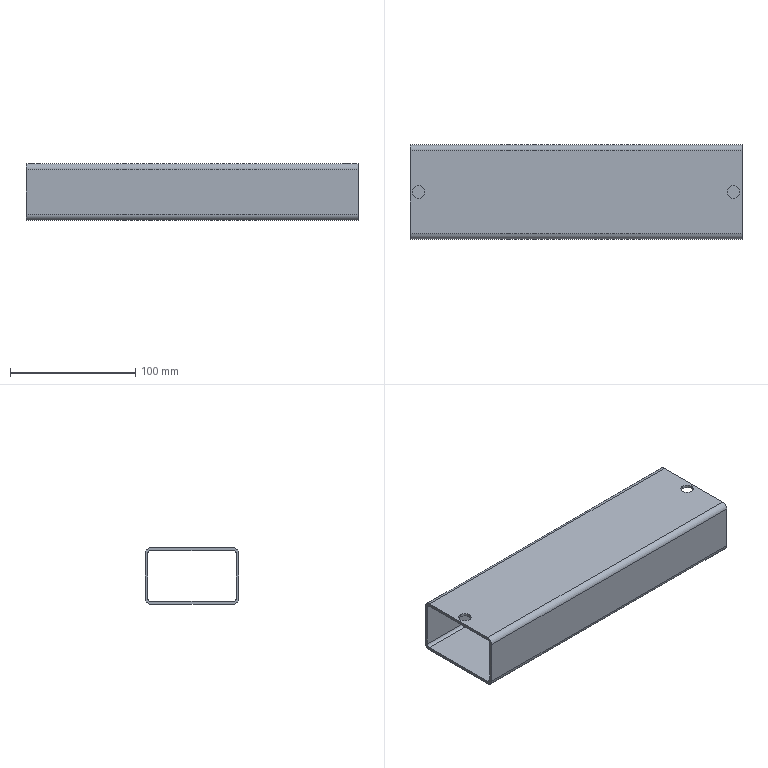Part | STEP file | [05]-1 | 1 solid | 22 faces | box 265 x 75 x 45 mm | volume 136701 mm3 | cylinder 12 | plane 10 | commonest cylinder face diameters 4.6 x4 9.2 x4 10 x4
STEP:
#1=CARTESIAN_POINT('',(278.,42.5,45.));
#2=VERTEX_POINT('',#1);
#3=CARTESIAN_POINT('',(278.,32.5,45.));
#4=VERTEX_POINT('',#3);
#5=CARTESIAN_POINT('',(278.,37.5,45.));
#6=DIRECTION('',(0.,0.,-1.));
#7=DIRECTION('',(0.,-1.,0.));
#8=AXIS2_PLACEMENT_3D('',#5,#6,#7);
#9=CIRCLE('',#8,5.);
#10=EDGE_CURVE('',#2,#4,#9,.T.);
#11=ORIENTED_EDGE('',*,*,#10,.F.);
#12=CARTESIAN_POINT('',(278.,42.5,42.7));
#13=VERTEX_POINT('',#12);
#14=CARTESIAN_POINT('',(278.,42.5,45.));
#15=DIRECTION('',(0.,0.,-1.));
#16=VECTOR('',#15,1000.);
#17=LINE('',#14,#16);
#18=EDGE_CURVE('',#2,#13,#17,.T.);
#19=ORIENTED_EDGE('',*,*,#18,.T.);
#20=CARTESIAN_POINT('',(278.,32.5,42.7));
#21=VERTEX_POINT('',#20);
#22=CARTESIAN_POINT('',(278.,37.5,42.7));
#23=DIRECTION('',(0.,0.,1.));
#24=DIRECTION('',(0.,1.,0.));
#25=AXIS2_PLACEMENT_3D('',#22,#23,#24);
#26=CIRCLE('',#25,5.);
#27=EDGE_CURVE('',#21,#13,#26,.T.);
#28=ORIENTED_EDGE('',*,*,#27,.F.);
#29=CARTESIAN_POINT('',(278.,32.5,45.));
#30=DIRECTION('',(0.,0.,-1.));
#31=VECTOR('',#30,1000.);
#32=LINE('',#29,#31);
#33=EDGE_CURVE('',#4,#21,#32,.T.);
#34=ORIENTED_EDGE('',*,*,#33,.F.);
#35=EDGE_LOOP('',(#11,#19,#28,#34));
#36=FACE_OUTER_BOUND('',#35,.T.);
#37=CARTESIAN_POINT('',(278.,37.5,45.));
#38=DIRECTION('',(0.,0.,-1.));
#39=DIRECTION('',(0.,-1.,0.));
#40=AXIS2_PLACEMENT_3D('',#37,#38,#39);
#41=CYLINDRICAL_SURFACE('',#40,5.);
#42=ADVANCED_FACE('',(#36),#41,.F.);
#43=CARTESIAN_POINT('',(27.,42.5,45.));
#44=VERTEX_POINT('',#43);
#45=CARTESIAN_POINT('',(27.,32.5,45.));
#46=VERTEX_POINT('',#45);
#47=CARTESIAN_POINT('',(27.,37.5,45.));
#48=DIRECTION('',(0.,0.,-1.));
#49=DIRECTION('',(0.,-1.,0.));
#50=AXIS2_PLACEMENT_3D('',#47,#48,#49);
#51=CIRCLE('',#50,5.);
#52=EDGE_CURVE('',#44,#46,#51,.T.);
#53=ORIENTED_EDGE('',*,*,#52,.F.);
#54=CARTESIAN_POINT('',(27.,42.5,42.7));
#55=VERTEX_POINT('',#54);
#56=CARTESIAN_POINT('',(27.,42.5,45.));
#57=DIRECTION('',(0.,0.,-1.));
#58=VECTOR('',#57,1000.);
#59=LINE('',#56,#58);
#60=EDGE_CURVE('',#44,#55,#59,.T.);
#61=ORIENTED_EDGE('',*,*,#60,.T.);
#62=CARTESIAN_POINT('',(27.,32.5,42.7));
#63=VERTEX_POINT('',#62);
#64=CARTESIAN_POINT('',(27.,37.5,42.7));
#65=DIRECTION('',(0.,0.,1.));
#66=DIRECTION('',(0.,1.,0.));
#67=AXIS2_PLACEMENT_3D('',#64,#65,#66);
#68=CIRCLE('',#67,5.);
#69=EDGE_CURVE('',#63,#55,#68,.T.);
#70=ORIENTED_EDGE('',*,*,#69,.F.);
#71=CARTESIAN_POINT('',(27.,32.5,45.));
#72=DIRECTION('',(0.,0.,-1.));
#73=VECTOR('',#72,1000.);
#74=LINE('',#71,#73);
#75=EDGE_CURVE('',#46,#63,#74,.T.);
#76=ORIENTED_EDGE('',*,*,#75,.F.);
#77=EDGE_LOOP('',(#53,#61,#70,#76));
#78=FACE_OUTER_BOUND('',#77,.T.);
#79=CARTESIAN_POINT('',(27.,37.5,45.));
#80=DIRECTION('',(0.,0.,-1.));
#81=DIRECTION('',(0.,-1.,0.));
#82=AXIS2_PLACEMENT_3D('',#79,#80,#81);
#83=CYLINDRICAL_SURFACE('',#82,5.);
#84=ADVANCED_FACE('',(#78),#83,.F.);
#85=CARTESIAN_POINT('',(20.,70.4,0.));
#86=VERTEX_POINT('',#85);
#87=CARTESIAN_POINT('',(20.,4.6,0.));
#88=VERTEX_POINT('',#87);
#89=CARTESIAN_POINT('',(20.,70.4,0.));
#90=DIRECTION('',(0.,-1.,0.));
#91=VECTOR('',#90,1000.);
#92=LINE('',#89,#91);
#93=EDGE_CURVE('',#86,#88,#92,.T.);
#94=ORIENTED_EDGE('',*,*,#93,.T.);
#95=CARTESIAN_POINT('',(20.,0.,4.6));
#96=VERTEX_POINT('',#95);
#97=CARTESIAN_POINT('',(20.,4.6,4.6));
#98=DIRECTION('',(-1.,0.,0.));
#99=DIRECTION('',(0.,0.,-1.));
#100=AXIS2_PLACEMENT_3D('',#97,#98,#99);
#101=CIRCLE('',#100,4.6);
#102=EDGE_CURVE('',#88,#96,#101,.T.);
#103=ORIENTED_EDGE('',*,*,#102,.T.);
#104=CARTESIAN_POINT('',(20.,0.,40.4));
#105=VERTEX_POINT('',#104);
#106=CARTESIAN_POINT('',(20.,0.,4.6));
#107=DIRECTION('',(0.,0.,1.));
#108=VECTOR('',#107,1000.);
#109=LINE('',#106,#108);
#110=EDGE_CURVE('',#96,#105,#109,.T.);
#111=ORIENTED_EDGE('',*,*,#110,.T.);
#112=CARTESIAN_POINT('',(20.,4.6,45.));
#113=VERTEX_POINT('',#112);
#114=CARTESIAN_POINT('',(20.,4.6,40.4));
#115=DIRECTION('',(-1.,0.,0.));
#116=DIRECTION('',(0.,0.,-1.));
#117=AXIS2_PLACEMENT_3D('',#114,#115,#116);
#118=CIRCLE('',#117,4.6);
#119=EDGE_CURVE('',#105,#113,#118,.T.);
#120=ORIENTED_EDGE('',*,*,#119,.T.);
#121=CARTESIAN_POINT('',(20.,70.4,45.));
#122=VERTEX_POINT('',#121);
#123=CARTESIAN_POINT('',(20.,4.6,45.));
#124=DIRECTION('',(0.,1.,0.));
#125=VECTOR('',#124,1000.);
#126=LINE('',#123,#125);
#127=EDGE_CURVE('',#113,#122,#126,.T.);
#128=ORIENTED_EDGE('',*,*,#127,.T.);
#129=CARTESIAN_POINT('',(20.,75.,40.4));
#130=VERTEX_POINT('',#129);
#131=CARTESIAN_POINT('',(20.,70.4,40.4));
#132=DIRECTION('',(-1.,0.,0.));
#133=DIRECTION('',(0.,0.,-1.));
#134=AXIS2_PLACEMENT_3D('',#131,#132,#133);
#135=CIRCLE('',#134,4.6);
#136=EDGE_CURVE('',#122,#130,#135,.T.);
#137=ORIENTED_EDGE('',*,*,#136,.T.);
#138=CARTESIAN_POINT('',(20.,75.,4.6));
#139=VERTEX_POINT('',#138);
#140=CARTESIAN_POINT('',(20.,75.,40.4));
#141=DIRECTION('',(0.,0.,-1.));
#142=VECTOR('',#141,1000.);
#143=LINE('',#140,#142);
#144=EDGE_CURVE('',#130,#139,#143,.T.);
#145=ORIENTED_EDGE('',*,*,#144,.T.);
#146=CARTESIAN_POINT('',(20.,70.4,4.6));
#147=DIRECTION('',(-1.,0.,0.));
#148=DIRECTION('',(0.,0.,-1.));
#149=AXIS2_PLACEMENT_3D('',#146,#147,#148);
#150=CIRCLE('',#149,4.6);
#151=EDGE_CURVE('',#139,#86,#150,.T.);
#152=ORIENTED_EDGE('',*,*,#151,.T.);
#153=EDGE_LOOP('',(#94,#103,#111,#120,#128,#137,#145,#152));
#154=FACE_OUTER_BOUND('',#153,.T.);
#155=CARTESIAN_POINT('',(20.,70.4,2.3));
#156=VERTEX_POINT('',#155);
#157=CARTESIAN_POINT('',(20.,4.6,2.3));
#158=VERTEX_POINT('',#157);
#159=CARTESIAN_POINT('',(20.,70.4,2.3));
#160=DIRECTION('',(0.,-1.,0.));
#161=VECTOR('',#160,1000.);
#162=LINE('',#159,#161);
#163=EDGE_CURVE('',#156,#158,#162,.T.);
#164=ORIENTED_EDGE('',*,*,#163,.F.);
#165=CARTESIAN_POINT('',(20.,72.7,4.6));
#166=VERTEX_POINT('',#165);
#167=CARTESIAN_POINT('',(20.,70.4,4.6));
#168=DIRECTION('',(-1.,0.,0.));
#169=DIRECTION('',(0.,1.,0.));
#170=AXIS2_PLACEMENT_3D('',#167,#168,#169);
#171=CIRCLE('',#170,2.3);
#172=EDGE_CURVE('',#166,#156,#171,.T.);
#173=ORIENTED_EDGE('',*,*,#172,.F.);
#174=CARTESIAN_POINT('',(20.,72.7,40.4));
#175=VERTEX_POINT('',#174);
#176=CARTESIAN_POINT('',(20.,72.7,40.4));
#177=DIRECTION('',(0.,0.,-1.));
#178=VECTOR('',#177,1000.);
#179=LINE('',#176,#178);
#180=EDGE_CURVE('',#175,#166,#179,.T.);
#181=ORIENTED_EDGE('',*,*,#180,.F.);
#182=CARTESIAN_POINT('',(20.,70.4,42.7));
#183=VERTEX_POINT('',#182);
#184=CARTESIAN_POINT('',(20.,70.4,40.4));
#185=DIRECTION('',(-1.,0.,0.));
#186=DIRECTION('',(0.,1.,0.));
#187=AXIS2_PLACEMENT_3D('',#184,#185,#186);
#188=CIRCLE('',#187,2.3);
#189=EDGE_CURVE('',#183,#175,#188,.T.);
#190=ORIENTED_EDGE('',*,*,#189,.F.);
#191=CARTESIAN_POINT('',(20.,4.6,42.7));
#192=VERTEX_POINT('',#191);
#193=CARTESIAN_POINT('',(20.,4.6,42.7));
#194=DIRECTION('',(0.,1.,0.));
#195=VECTOR('',#194,1000.);
#196=LINE('',#193,#195);
#197=EDGE_CURVE('',#192,#183,#196,.T.);
#198=ORIENTED_EDGE('',*,*,#197,.F.);
#199=CARTESIAN_POINT('',(20.,2.3,40.4));
#200=VERTEX_POINT('',#199);
#201=CARTESIAN_POINT('',(20.,4.6,40.4));
#202=DIRECTION('',(-1.,0.,0.));
#203=DIRECTION('',(0.,1.,0.));
#204=AXIS2_PLACEMENT_3D('',#201,#202,#203);
#205=CIRCLE('',#204,2.3);
#206=EDGE_CURVE('',#200,#192,#205,.T.);
#207=ORIENTED_EDGE('',*,*,#206,.F.);
#208=CARTESIAN_POINT('',(20.,2.3,4.6));
#209=VERTEX_POINT('',#208);
#210=CARTESIAN_POINT('',(20.,2.3,4.6));
#211=DIRECTION('',(0.,0.,1.));
#212=VECTOR('',#211,1000.);
#213=LINE('',#210,#212);
#214=EDGE_CURVE('',#209,#200,#213,.T.);
#215=ORIENTED_EDGE('',*,*,#214,.F.);
#216=CARTESIAN_POINT('',(20.,4.6,4.6));
#217=DIRECTION('',(-1.,0.,0.));
#218=DIRECTION('',(0.,1.,0.));
#219=AXIS2_PLACEMENT_3D('',#216,#217,#218);
#220=CIRCLE('',#219,2.3);
#221=EDGE_CURVE('',#158,#209,#220,.T.);
#222=ORIENTED_EDGE('',*,*,#221,.F.);
#223=EDGE_LOOP('',(#164,#173,#181,#190,#198,#207,#215,#222));
#224=FACE_BOUND('',#223,.T.);
#225=CARTESIAN_POINT('',(20.,4.6,4.6));
#226=DIRECTION('',(-1.,0.,0.));
#227=DIRECTION('',(0.,0.,-1.));
#228=AXIS2_PLACEMENT_3D('',#225,#226,#227);
#229=PLANE('',#228);
#230=ADVANCED_FACE('',(#154,#224),#229,.T.);
#231=CARTESIAN_POINT('',(285.,70.4,0.));
#232=VERTEX_POINT('',#231);
#233=CARTESIAN_POINT('',(285.,4.6,0.));
#234=VERTEX_POINT('',#233);
#235=CARTESIAN_POINT('',(285.,70.4,0.));
#236=DIRECTION('',(0.,-1.,0.));
#237=VECTOR('',#236,1000.);
#238=LINE('',#235,#237);
#239=EDGE_CURVE('',#232,#234,#238,.T.);
#240=ORIENTED_EDGE('',*,*,#239,.F.);
#241=CARTESIAN_POINT('',(285.,75.,4.6));
#242=VERTEX_POINT('',#241);
#243=CARTESIAN_POINT('',(285.,70.4,4.6));
#244=DIRECTION('',(-1.,0.,0.));
#245=DIRECTION('',(0.,0.,-1.));
#246=AXIS2_PLACEMENT_3D('',#243,#244,#245);
#247=CIRCLE('',#246,4.6);
#248=EDGE_CURVE('',#242,#232,#247,.T.);
#249=ORIENTED_EDGE('',*,*,#248,.F.);
#250=CARTESIAN_POINT('',(285.,75.,40.4));
#251=VERTEX_POINT('',#250);
#252=CARTESIAN_POINT('',(285.,75.,40.4));
#253=DIRECTION('',(0.,0.,-1.));
#254=VECTOR('',#253,1000.);
#255=LINE('',#252,#254);
#256=EDGE_CURVE('',#251,#242,#255,.T.);
#257=ORIENTED_EDGE('',*,*,#256,.F.);
#258=CARTESIAN_POINT('',(285.,70.4,45.));
#259=VERTEX_POINT('',#258);
#260=CARTESIAN_POINT('',(285.,70.4,40.4));
#261=DIRECTION('',(-1.,0.,0.));
#262=DIRECTION('',(0.,0.,-1.));
#263=AXIS2_PLACEMENT_3D('',#260,#261,#262);
#264=CIRCLE('',#263,4.6);
#265=EDGE_CURVE('',#259,#251,#264,.T.);
#266=ORIENTED_EDGE('',*,*,#265,.F.);
#267=CARTESIAN_POINT('',(285.,4.6,45.));
#268=VERTEX_POINT('',#267);
#269=CARTESIAN_POINT('',(285.,4.6,45.));
#270=DIRECTION('',(0.,1.,0.));
#271=VECTOR('',#270,1000.);
#272=LINE('',#269,#271);
#273=EDGE_CURVE('',#268,#259,#272,.T.);
#274=ORIENTED_EDGE('',*,*,#273,.F.);
#275=CARTESIAN_POINT('',(285.,0.,40.4));
#276=VERTEX_POINT('',#275);
#277=CARTESIAN_POINT('',(285.,4.6,40.4));
#278=DIRECTION('',(-1.,0.,0.));
#279=DIRECTION('',(0.,0.,-1.));
#280=AXIS2_PLACEMENT_3D('',#277,#278,#279);
#281=CIRCLE('',#280,4.6);
#282=EDGE_CURVE('',#276,#268,#281,.T.);
#283=ORIENTED_EDGE('',*,*,#282,.F.);
#284=CARTESIAN_POINT('',(285.,0.,4.6));
#285=VERTEX_POINT('',#284);
#286=CARTESIAN_POINT('',(285.,0.,4.6));
#287=DIRECTION('',(0.,0.,1.));
#288=VECTOR('',#287,1000.);
#289=LINE('',#286,#288);
#290=EDGE_CURVE('',#285,#276,#289,.T.);
#291=ORIENTED_EDGE('',*,*,#290,.F.);
#292=CARTESIAN_POINT('',(285.,4.6,4.6));
#293=DIRECTION('',(-1.,0.,0.));
#294=DIRECTION('',(0.,0.,-1.));
#295=AXIS2_PLACEMENT_3D('',#292,#293,#294);
#296=CIRCLE('',#295,4.6);
#297=EDGE_CURVE('',#234,#285,#296,.T.);
#298=ORIENTED_EDGE('',*,*,#297,.F.);
#299=EDGE_LOOP('',(#240,#249,#257,#266,#274,#283,#291,#298));
#300=FACE_OUTER_BOUND('',#299,.T.);
#301=CARTESIAN_POINT('',(285.,72.7,4.6));
#302=VERTEX_POINT('',#301);
#303=CARTESIAN_POINT('',(285.,70.4,2.3));
#304=VERTEX_POINT('',#303);
#305=CARTESIAN_POINT('',(285.,70.4,4.6));
#306=DIRECTION('',(-1.,0.,0.));
#307=DIRECTION('',(0.,1.,0.));
#308=AXIS2_PLACEMENT_3D('',#305,#306,#307);
#309=CIRCLE('',#308,2.3);
#310=EDGE_CURVE('',#302,#304,#309,.T.);
#311=ORIENTED_EDGE('',*,*,#310,.T.);
#312=CARTESIAN_POINT('',(285.,4.6,2.3));
#313=VERTEX_POINT('',#312);
#314=CARTESIAN_POINT('',(285.,70.4,2.3));
#315=DIRECTION('',(0.,-1.,0.));
#316=VECTOR('',#315,1000.);
#317=LINE('',#314,#316);
#318=EDGE_CURVE('',#304,#313,#317,.T.);
#319=ORIENTED_EDGE('',*,*,#318,.T.);
#320=CARTESIAN_POINT('',(285.,2.3,4.6));
#321=VERTEX_POINT('',#320);
#322=CARTESIAN_POINT('',(285.,4.6,4.6));
#323=DIRECTION('',(-1.,0.,0.));
#324=DIRECTION('',(0.,1.,0.));
#325=AXIS2_PLACEMENT_3D('',#322,#323,#324);
#326=CIRCLE('',#325,2.3);
#327=EDGE_CURVE('',#313,#321,#326,.T.);
#328=ORIENTED_EDGE('',*,*,#327,.T.);
#329=CARTESIAN_POINT('',(285.,2.3,40.4));
#330=VERTEX_POINT('',#329);
#331=CARTESIAN_POINT('',(285.,2.3,4.6));
#332=DIRECTION('',(0.,0.,1.));
#333=VECTOR('',#332,1000.);
#334=LINE('',#331,#333);
#335=EDGE_CURVE('',#321,#330,#334,.T.);
#336=ORIENTED_EDGE('',*,*,#335,.T.);
#337=CARTESIAN_POINT('',(285.,4.6,42.7));
#338=VERTEX_POINT('',#337);
#339=CARTESIAN_POINT('',(285.,4.6,40.4));
#340=DIRECTION('',(-1.,0.,0.));
#341=DIRECTION('',(0.,1.,0.));
#342=AXIS2_PLACEMENT_3D('',#339,#340,#341);
#343=CIRCLE('',#342,2.3);
#344=EDGE_CURVE('',#330,#338,#343,.T.);
#345=ORIENTED_EDGE('',*,*,#344,.T.);
#346=CARTESIAN_POINT('',(285.,70.4,42.7));
#347=VERTEX_POINT('',#346);
#348=CARTESIAN_POINT('',(285.,4.6,42.7));
#349=DIRECTION('',(0.,1.,0.));
#350=VECTOR('',#349,1000.);
#351=LINE('',#348,#350);
#352=EDGE_CURVE('',#338,#347,#351,.T.);
#353=ORIENTED_EDGE('',*,*,#352,.T.);
#354=CARTESIAN_POINT('',(285.,72.7,40.4));
#355=VERTEX_POINT('',#354);
#356=CARTESIAN_POINT('',(285.,70.4,40.4));
#357=DIRECTION('',(-1.,0.,0.));
#358=DIRECTION('',(0.,1.,0.));
#359=AXIS2_PLACEMENT_3D('',#356,#357,#358);
#360=CIRCLE('',#359,2.3);
#361=EDGE_CURVE('',#347,#355,#360,.T.);
#362=ORIENTED_EDGE('',*,*,#361,.T.);
#363=CARTESIAN_POINT('',(285.,72.7,40.4));
#364=DIRECTION('',(0.,0.,-1.));
#365=VECTOR('',#364,1000.);
#366=LINE('',#363,#365);
#367=EDGE_CURVE('',#355,#302,#366,.T.);
#368=ORIENTED_EDGE('',*,*,#367,.T.);
#369=EDGE_LOOP('',(#311,#319,#328,#336,#345,#353,#362,#368));
#370=FACE_BOUND('',#369,.T.);
#371=CARTESIAN_POINT('',(285.,4.6,4.6));
#372=DIRECTION('',(-1.,0.,0.));
#373=DIRECTION('',(0.,0.,-1.));
#374=AXIS2_PLACEMENT_3D('',#371,#372,#373);
#375=PLANE('',#374);
#376=ADVANCED_FACE('',(#300,#370),#375,.F.);
#377=ORIENTED_EDGE('',*,*,#239,.T.);
#378=CARTESIAN_POINT('',(20.,4.6,0.));
#379=DIRECTION('',(1.,0.,0.));
#380=VECTOR('',#379,1000.);
#381=LINE('',#378,#380);
#382=EDGE_CURVE('',#88,#234,#381,.T.);
#383=ORIENTED_EDGE('',*,*,#382,.F.);
#384=ORIENTED_EDGE('',*,*,#93,.F.);
#385=CARTESIAN_POINT('',(20.,70.4,0.));
#386=DIRECTION('',(1.,0.,0.));
#387=VECTOR('',#386,1000.);
#388=LINE('',#385,#387);
#389=EDGE_CURVE('',#86,#232,#388,.T.);
#390=ORIENTED_EDGE('',*,*,#389,.T.);
#391=EDGE_LOOP('',(#377,#383,#384,#390));
#392=FACE_OUTER_BOUND('',#391,.T.);
#393=CARTESIAN_POINT('',(20.,70.4,0.));
#394=DIRECTION('',(0.,0.,1.));
#395=DIRECTION('',(0.,1.,0.));
#396=AXIS2_PLACEMENT_3D('',#393,#394,#395);
#397=PLANE('',#396);
#398=ADVANCED_FACE('',(#392),#397,.F.);
#399=ORIENTED_EDGE('',*,*,#297,.T.);
#400=CARTESIAN_POINT('',(20.,0.,4.6));
#401=DIRECTION('',(1.,0.,0.));
#402=VECTOR('',#401,1000.);
#403=LINE('',#400,#402);
#404=EDGE_CURVE('',#96,#285,#403,.T.);
#405=ORIENTED_EDGE('',*,*,#404,.F.);
#406=ORIENTED_EDGE('',*,*,#102,.F.);
#407=ORIENTED_EDGE('',*,*,#382,.T.);
#408=EDGE_LOOP('',(#399,#405,#406,#407));
#409=FACE_OUTER_BOUND('',#408,.T.);
#410=CARTESIAN_POINT('',(20.,4.6,4.6));
#411=DIRECTION('',(1.,0.,0.));
#412=DIRECTION('',(0.,0.,1.));
#413=AXIS2_PLACEMENT_3D('',#410,#411,#412);
#414=CYLINDRICAL_SURFACE('',#413,4.6);
#415=ADVANCED_FACE('',(#409),#414,.T.);
#416=ORIENTED_EDGE('',*,*,#290,.T.);
#417=CARTESIAN_POINT('',(20.,0.,40.4));
#418=DIRECTION('',(1.,0.,0.));
#419=VECTOR('',#418,1000.);
#420=LINE('',#417,#419);
#421=EDGE_CURVE('',#105,#276,#420,.T.);
#422=ORIENTED_EDGE('',*,*,#421,.F.);
#423=ORIENTED_EDGE('',*,*,#110,.F.);
#424=ORIENTED_EDGE('',*,*,#404,.T.);
#425=EDGE_LOOP('',(#416,#422,#423,#424));
#426=FACE_OUTER_BOUND('',#425,.T.);
#427=CARTESIAN_POINT('',(20.,0.,4.6));
#428=DIRECTION('',(0.,1.,0.));
#429=DIRECTION('',(0.,0.,-1.));
#430=AXIS2_PLACEMENT_3D('',#427,#428,#429);
#431=PLANE('',#430);
#432=ADVANCED_FACE('',(#426),#431,.F.);
#433=ORIENTED_EDGE('',*,*,#282,.T.);
#434=CARTESIAN_POINT('',(20.,4.6,45.));
#435=DIRECTION('',(1.,0.,0.));
#436=VECTOR('',#435,1000.);
#437=LINE('',#434,#436);
#438=EDGE_CURVE('',#113,#268,#437,.T.);
#439=ORIENTED_EDGE('',*,*,#438,.F.);
#440=ORIENTED_EDGE('',*,*,#119,.F.);
#441=ORIENTED_EDGE('',*,*,#421,.T.);
#442=EDGE_LOOP('',(#433,#439,#440,#441));
#443=FACE_OUTER_BOUND('',#442,.T.);
#444=CARTESIAN_POINT('',(20.,4.6,40.4));
#445=DIRECTION('',(1.,0.,0.));
#446=DIRECTION('',(0.,0.,1.));
#447=AXIS2_PLACEMENT_3D('',#444,#445,#446);
#448=CYLINDRICAL_SURFACE('',#447,4.6);
#449=ADVANCED_FACE('',(#443),#448,.T.);
#450=CARTESIAN_POINT('',(278.,37.5,45.));
#451=DIRECTION('',(0.,0.,-1.));
#452=DIRECTION('',(0.,-1.,0.));
#453=AXIS2_PLACEMENT_3D('',#450,#451,#452);
#454=CIRCLE('',#453,5.);
#455=EDGE_CURVE('',#4,#2,#454,.T.);
#456=ORIENTED_EDGE('',*,*,#455,.T.);
#457=ORIENTED_EDGE('',*,*,#10,.T.);
#458=EDGE_LOOP('',(#456,#457));
#459=FACE_BOUND('',#458,.T.);
#460=CARTESIAN_POINT('',(27.,37.5,45.));
#461=DIRECTION('',(0.,0.,-1.));
#462=DIRECTION('',(0.,-1.,0.));
#463=AXIS2_PLACEMENT_3D('',#460,#461,#462);
#464=CIRCLE('',#463,5.);
#465=EDGE_CURVE('',#46,#44,#464,.T.);
#466=ORIENTED_EDGE('',*,*,#465,.T.);
#467=ORIENTED_EDGE('',*,*,#52,.T.);
#468=EDGE_LOOP('',(#466,#467));
#469=FACE_BOUND('',#468,.T.);
#470=ORIENTED_EDGE('',*,*,#273,.T.);
#471=CARTESIAN_POINT('',(20.,70.4,45.));
#472=DIRECTION('',(1.,0.,0.));
#473=VECTOR('',#472,1000.);
#474=LINE('',#471,#473);
#475=EDGE_CURVE('',#122,#259,#474,.T.);
#476=ORIENTED_EDGE('',*,*,#475,.F.);
#477=ORIENTED_EDGE('',*,*,#127,.F.);
#478=ORIENTED_EDGE('',*,*,#438,.T.);
#479=EDGE_LOOP('',(#470,#476,#477,#478));
#480=FACE_OUTER_BOUND('',#479,.T.);
#481=CARTESIAN_POINT('',(20.,4.6,45.));
#482=DIRECTION('',(0.,0.,-1.));
#483=DIRECTION('',(0.,-1.,0.));
#484=AXIS2_PLACEMENT_3D('',#481,#482,#483);
#485=PLANE('',#484);
#486=ADVANCED_FACE('',(#459,#469,#480),#485,.F.);
#487=ORIENTED_EDGE('',*,*,#265,.T.);
#488=CARTESIAN_POINT('',(20.,75.,40.4));
#489=DIRECTION('',(1.,0.,0.));
#490=VECTOR('',#489,1000.);
#491=LINE('',#488,#490);
#492=EDGE_CURVE('',#130,#251,#491,.T.);
#493=ORIENTED_EDGE('',*,*,#492,.F.);
#494=ORIENTED_EDGE('',*,*,#136,.F.);
#495=ORIENTED_EDGE('',*,*,#475,.T.);
#496=EDGE_LOOP('',(#487,#493,#494,#495));
#497=FACE_OUTER_BOUND('',#496,.T.);
#498=CARTESIAN_POINT('',(20.,70.4,40.4));
#499=DIRECTION('',(1.,0.,0.));
#500=DIRECTION('',(0.,0.,1.));
#501=AXIS2_PLACEMENT_3D('',#498,#499,#500);
#502=CYLINDRICAL_SURFACE('',#501,4.6);
#503=ADVANCED_FACE('',(#497),#502,.T.);
#504=ORIENTED_EDGE('',*,*,#256,.T.);
#505=CARTESIAN_POINT('',(20.,75.,4.6));
#506=DIRECTION('',(1.,0.,0.));
#507=VECTOR('',#506,1000.);
#508=LINE('',#505,#507);
#509=EDGE_CURVE('',#139,#242,#508,.T.);
#510=ORIENTED_EDGE('',*,*,#509,.F.);
#511=ORIENTED_EDGE('',*,*,#144,.F.);
#512=ORIENTED_EDGE('',*,*,#492,.T.);
#513=EDGE_LOOP('',(#504,#510,#511,#512));
#514=FACE_OUTER_BOUND('',#513,.T.);
#515=CARTESIAN_POINT('',(20.,75.,40.4));
#516=DIRECTION('',(0.,-1.,0.));
#517=DIRECTION('',(-1.,0.,0.));
#518=AXIS2_PLACEMENT_3D('',#515,#516,#517);
#519=PLANE('',#518);
#520=ADVANCED_FACE('',(#514),#519,.F.);
#521=ORIENTED_EDGE('',*,*,#248,.T.);
#522=ORIENTED_EDGE('',*,*,#389,.F.);
#523=ORIENTED_EDGE('',*,*,#151,.F.);
#524=ORIENTED_EDGE('',*,*,#509,.T.);
#525=EDGE_LOOP('',(#521,#522,#523,#524));
#526=FACE_OUTER_BOUND('',#525,.T.);
#527=CARTESIAN_POINT('',(20.,70.4,4.6));
#528=DIRECTION('',(1.,0.,0.));
#529=DIRECTION('',(0.,0.,1.));
#530=AXIS2_PLACEMENT_3D('',#527,#528,#529);
#531=CYLINDRICAL_SURFACE('',#530,4.6);
#532=ADVANCED_FACE('',(#526),#531,.T.);
#533=ORIENTED_EDGE('',*,*,#310,.F.);
#534=CARTESIAN_POINT('',(20.,72.7,4.6));
#535=DIRECTION('',(1.,0.,0.));
#536=VECTOR('',#535,1000.);
#537=LINE('',#534,#536);
#538=EDGE_CURVE('',#166,#302,#537,.T.);
#539=ORIENTED_EDGE('',*,*,#538,.F.);
#540=ORIENTED_EDGE('',*,*,#172,.T.);
#541=CARTESIAN_POINT('',(20.,70.4,2.3));
#542=DIRECTION('',(1.,0.,0.));
#543=VECTOR('',#542,1000.);
#544=LINE('',#541,#543);
#545=EDGE_CURVE('',#156,#304,#544,.T.);
#546=ORIENTED_EDGE('',*,*,#545,.T.);
#547=EDGE_LOOP('',(#533,#539,#540,#546));
#548=FACE_OUTER_BOUND('',#547,.T.);
#549=CARTESIAN_POINT('',(20.,70.4,4.6));
#550=DIRECTION('',(1.,0.,0.));
#551=DIRECTION('',(0.,-1.,0.));
#552=AXIS2_PLACEMENT_3D('',#549,#550,#551);
#553=CYLINDRICAL_SURFACE('',#552,2.3);
#554=ADVANCED_FACE('',(#548),#553,.F.);
#555=ORIENTED_EDGE('',*,*,#318,.F.);
#556=ORIENTED_EDGE('',*,*,#545,.F.);
#557=ORIENTED_EDGE('',*,*,#163,.T.);
#558=CARTESIAN_POINT('',(20.,4.6,2.3));
#559=DIRECTION('',(1.,0.,0.));
#560=VECTOR('',#559,1000.);
#561=LINE('',#558,#560);
#562=EDGE_CURVE('',#158,#313,#561,.T.);
#563=ORIENTED_EDGE('',*,*,#562,.T.);
#564=EDGE_LOOP('',(#555,#556,#557,#563));
#565=FACE_OUTER_BOUND('',#564,.T.);
#566=CARTESIAN_POINT('',(20.,70.4,2.3));
#567=DIRECTION('',(0.,0.,1.));
#568=DIRECTION('',(1.,0.,0.));
#569=AXIS2_PLACEMENT_3D('',#566,#567,#568);
#570=PLANE('',#569);
#571=ADVANCED_FACE('',(#565),#570,.T.);
#572=ORIENTED_EDGE('',*,*,#327,.F.);
#573=ORIENTED_EDGE('',*,*,#562,.F.);
#574=ORIENTED_EDGE('',*,*,#221,.T.);
#575=CARTESIAN_POINT('',(20.,2.3,4.6));
#576=DIRECTION('',(1.,0.,0.));
#577=VECTOR('',#576,1000.);
#578=LINE('',#575,#577);
#579=EDGE_CURVE('',#209,#321,#578,.T.);
#580=ORIENTED_EDGE('',*,*,#579,.T.);
#581=EDGE_LOOP('',(#572,#573,#574,#580));
#582=FACE_OUTER_BOUND('',#581,.T.);
#583=CARTESIAN_POINT('',(20.,4.6,4.6));
#584=DIRECTION('',(1.,0.,0.));
#585=DIRECTION('',(0.,-1.,0.));
#586=AXIS2_PLACEMENT_3D('',#583,#584,#585);
#587=CYLINDRICAL_SURFACE('',#586,2.3);
#588=ADVANCED_FACE('',(#582),#587,.F.);
#589=ORIENTED_EDGE('',*,*,#335,.F.);
#590=ORIENTED_EDGE('',*,*,#579,.F.);
#591=ORIENTED_EDGE('',*,*,#214,.T.);
#592=CARTESIAN_POINT('',(20.,2.3,40.4));
#593=DIRECTION('',(1.,0.,0.));
#594=VECTOR('',#593,1000.);
#595=LINE('',#592,#594);
#596=EDGE_CURVE('',#200,#330,#595,.T.);
#597=ORIENTED_EDGE('',*,*,#596,.T.);
#598=EDGE_LOOP('',(#589,#590,#591,#597));
#599=FACE_OUTER_BOUND('',#598,.T.);
#600=CARTESIAN_POINT('',(20.,2.3,4.6));
#601=DIRECTION('',(0.,1.,0.));
#602=DIRECTION('',(1.,0.,0.));
#603=AXIS2_PLACEMENT_3D('',#600,#601,#602);
#604=PLANE('',#603);
#605=ADVANCED_FACE('',(#599),#604,.T.);
#606=ORIENTED_EDGE('',*,*,#344,.F.);
#607=ORIENTED_EDGE('',*,*,#596,.F.);
#608=ORIENTED_EDGE('',*,*,#206,.T.);
#609=CARTESIAN_POINT('',(20.,4.6,42.7));
#610=DIRECTION('',(1.,0.,0.));
#611=VECTOR('',#610,1000.);
#612=LINE('',#609,#611);
#613=EDGE_CURVE('',#192,#338,#612,.T.);
#614=ORIENTED_EDGE('',*,*,#613,.T.);
#615=EDGE_LOOP('',(#606,#607,#608,#614));
#616=FACE_OUTER_BOUND('',#615,.T.);
#617=CARTESIAN_POINT('',(20.,4.6,40.4));
#618=DIRECTION('',(1.,0.,0.));
#619=DIRECTION('',(0.,-1.,0.));
#620=AXIS2_PLACEMENT_3D('',#617,#618,#619);
#621=CYLINDRICAL_SURFACE('',#620,2.3);
#622=ADVANCED_FACE('',(#616),#621,.F.);
#623=ORIENTED_EDGE('',*,*,#27,.T.);
#624=CARTESIAN_POINT('',(278.,37.5,42.7));
#625=DIRECTION('',(0.,0.,1.));
#626=DIRECTION('',(0.,1.,0.));
#627=AXIS2_PLACEMENT_3D('',#624,#625,#626);
#628=CIRCLE('',#627,5.);
#629=EDGE_CURVE('',#13,#21,#628,.T.);
#630=ORIENTED_EDGE('',*,*,#629,.T.);
#631=EDGE_LOOP('',(#623,#630));
#632=FACE_BOUND('',#631,.T.);
#633=ORIENTED_EDGE('',*,*,#69,.T.);
#634=CARTESIAN_POINT('',(27.,37.5,42.7));
#635=DIRECTION('',(0.,0.,1.));
#636=DIRECTION('',(0.,1.,0.));
#637=AXIS2_PLACEMENT_3D('',#634,#635,#636);
#638=CIRCLE('',#637,5.);
#639=EDGE_CURVE('',#55,#63,#638,.T.);
#640=ORIENTED_EDGE('',*,*,#639,.T.);
#641=EDGE_LOOP('',(#633,#640));
#642=FACE_BOUND('',#641,.T.);
#643=ORIENTED_EDGE('',*,*,#352,.F.);
#644=ORIENTED_EDGE('',*,*,#613,.F.);
#645=ORIENTED_EDGE('',*,*,#197,.T.);
#646=CARTESIAN_POINT('',(20.,70.4,42.7));
#647=DIRECTION('',(1.,0.,0.));
#648=VECTOR('',#647,1000.);
#649=LINE('',#646,#648);
#650=EDGE_CURVE('',#183,#347,#649,.T.);
#651=ORIENTED_EDGE('',*,*,#650,.T.);
#652=EDGE_LOOP('',(#643,#644,#645,#651));
#653=FACE_OUTER_BOUND('',#652,.T.);
#654=CARTESIAN_POINT('',(20.,4.6,42.7));
#655=DIRECTION('',(0.,0.,-1.));
#656=DIRECTION('',(0.,-1.,0.));
#657=AXIS2_PLACEMENT_3D('',#654,#655,#656);
#658=PLANE('',#657);
#659=ADVANCED_FACE('',(#632,#642,#653),#658,.T.);
#660=ORIENTED_EDGE('',*,*,#361,.F.);
#661=ORIENTED_EDGE('',*,*,#650,.F.);
#662=ORIENTED_EDGE('',*,*,#189,.T.);
#663=CARTESIAN_POINT('',(20.,72.7,40.4));
#664=DIRECTION('',(1.,0.,0.));
#665=VECTOR('',#664,1000.);
#666=LINE('',#663,#665);
#667=EDGE_CURVE('',#175,#355,#666,.T.);
#668=ORIENTED_EDGE('',*,*,#667,.T.);
#669=EDGE_LOOP('',(#660,#661,#662,#668));
#670=FACE_OUTER_BOUND('',#669,.T.);
#671=CARTESIAN_POINT('',(20.,70.4,40.4));
#672=DIRECTION('',(1.,0.,0.));
#673=DIRECTION('',(0.,-1.,0.));
#674=AXIS2_PLACEMENT_3D('',#671,#672,#673);
#675=CYLINDRICAL_SURFACE('',#674,2.3);
#676=ADVANCED_FACE('',(#670),#675,.F.);
#677=ORIENTED_EDGE('',*,*,#367,.F.);
#678=ORIENTED_EDGE('',*,*,#667,.F.);
#679=ORIENTED_EDGE('',*,*,#180,.T.);
#680=ORIENTED_EDGE('',*,*,#538,.T.);
#681=EDGE_LOOP('',(#677,#678,#679,#680));
#682=FACE_OUTER_BOUND('',#681,.T.);
#683=CARTESIAN_POINT('',(20.,72.7,40.4));
#684=DIRECTION('',(0.,-1.,0.));
#685=DIRECTION('',(0.,0.,1.));
#686=AXIS2_PLACEMENT_3D('',#683,#684,#685);
#687=PLANE('',#686);
#688=ADVANCED_FACE('',(#682),#687,.T.);
#689=ORIENTED_EDGE('',*,*,#60,.F.);
#690=ORIENTED_EDGE('',*,*,#465,.F.);
#691=ORIENTED_EDGE('',*,*,#75,.T.);
#692=ORIENTED_EDGE('',*,*,#639,.F.);
#693=EDGE_LOOP('',(#689,#690,#691,#692));
#694=FACE_OUTER_BOUND('',#693,.T.);
#695=CARTESIAN_POINT('',(27.,37.5,45.));
#696=DIRECTION('',(0.,0.,-1.));
#697=DIRECTION('',(0.,-1.,0.));
#698=AXIS2_PLACEMENT_3D('',#695,#696,#697);
#699=CYLINDRICAL_SURFACE('',#698,5.);
#700=ADVANCED_FACE('',(#694),#699,.F.);
#701=ORIENTED_EDGE('',*,*,#18,.F.);
#702=ORIENTED_EDGE('',*,*,#455,.F.);
#703=ORIENTED_EDGE('',*,*,#33,.T.);
#704=ORIENTED_EDGE('',*,*,#629,.F.);
#705=EDGE_LOOP('',(#701,#702,#703,#704));
#706=FACE_OUTER_BOUND('',#705,.T.);
#707=CARTESIAN_POINT('',(278.,37.5,45.));
#708=DIRECTION('',(0.,0.,-1.));
#709=DIRECTION('',(0.,-1.,0.));
#710=AXIS2_PLACEMENT_3D('',#707,#708,#709);
#711=CYLINDRICAL_SURFACE('',#710,5.);
#712=ADVANCED_FACE('',(#706),#711,.F.);
#713=CLOSED_SHELL('',(#42,#84,#230,#376,#398,#415,#432,#449,#486,#503,#520,#532,#554,#571,#588,#605,#622,#659,#676,#688,#700,#712));
#714=MANIFOLD_SOLID_BREP('',#713);
#715=CARTESIAN_POINT('',(0.,0.,0.));
#716=DIRECTION('',(0.,0.,1.));
#717=DIRECTION('',(1.,0.,0.));
#718=AXIS2_PLACEMENT_3D('',#715,#716,#717);
#719=(LENGTH_UNIT()NAMED_UNIT(*)SI_UNIT(.MILLI.,.METRE.));
#720=UNCERTAINTY_MEASURE_WITH_UNIT(LENGTH_MEASURE(0.00001),#719,'','');
#721=(NAMED_UNIT(*)PLANE_ANGLE_UNIT()SI_UNIT($,.RADIAN.));
#722=(NAMED_UNIT(*)SI_UNIT($,.STERADIAN.)SOLID_ANGLE_UNIT());
#723=(GEOMETRIC_REPRESENTATION_CONTEXT(3)GLOBAL_UNCERTAINTY_ASSIGNED_CONTEXT((#720))GLOBAL_UNIT_ASSIGNED_CONTEXT((#719,#721,#722))REPRESENTATION_CONTEXT('',''));
#724=ADVANCED_BREP_SHAPE_REPRESENTATION('',(#714,#718),#723);